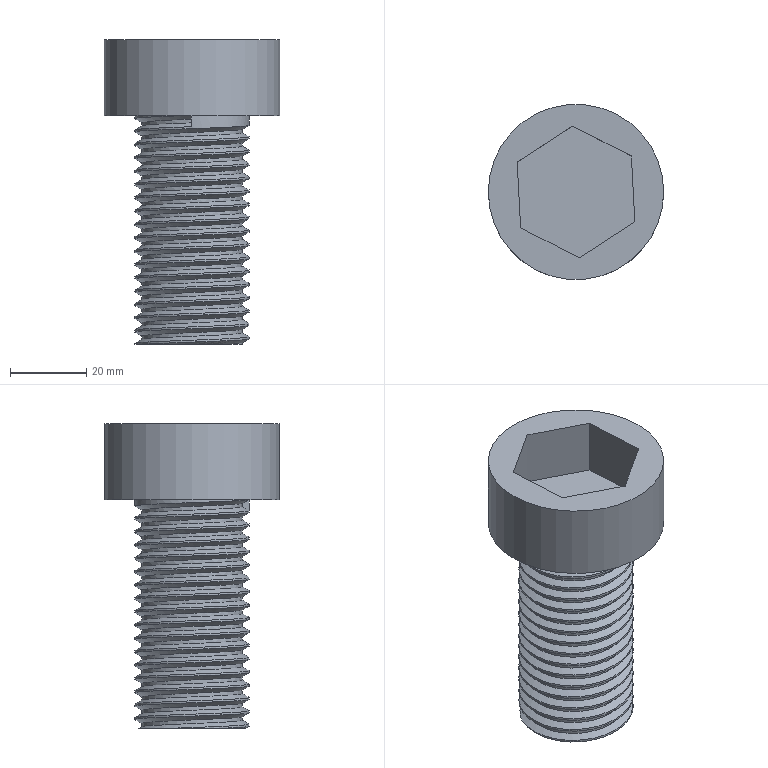Part | NX | features DATUM_CSYS 4, EXTRUDE 3, SKETCH 3, THREADS 1 | 1 solid | 17 faces | box 46 x 46 x 80 mm | volume 58631 mm3 | plane 11 | cylinder 3 | spline 3 | commonest cylinder face diameters 26.5 x1 30 x1 46 x1